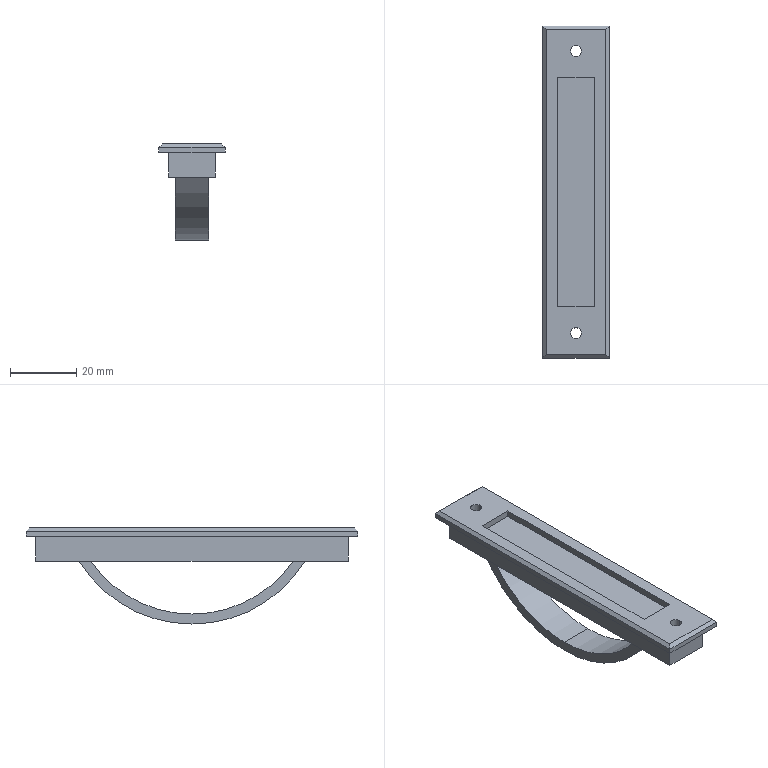Part | STEP file | XAC22-100 | 1 solid | 29 faces | box 20 x 100 x 28.929 mm | volume 15353 mm3 | plane 22 | cylinder 7 | commonest cylinder face diameters 3.3 x4 74 x2 80 x1